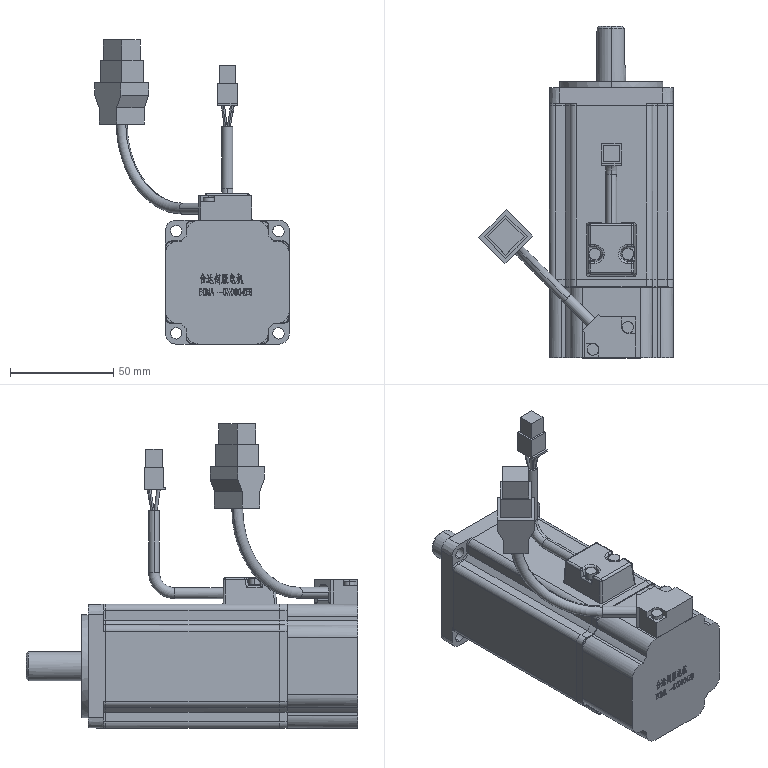Part | 1 solid | 1208 faces | box 94.241 x 160.703 x 147.367 mm | volume 450396 mm3 | plane 735 | spline 265 | cylinder 161 | cone 26 | torus 11 | sphere 10 | commonest cylinder face diameters 6 x39 2 x20 5.5 x16 0.6 x12 1.5 x11 5.3 x8